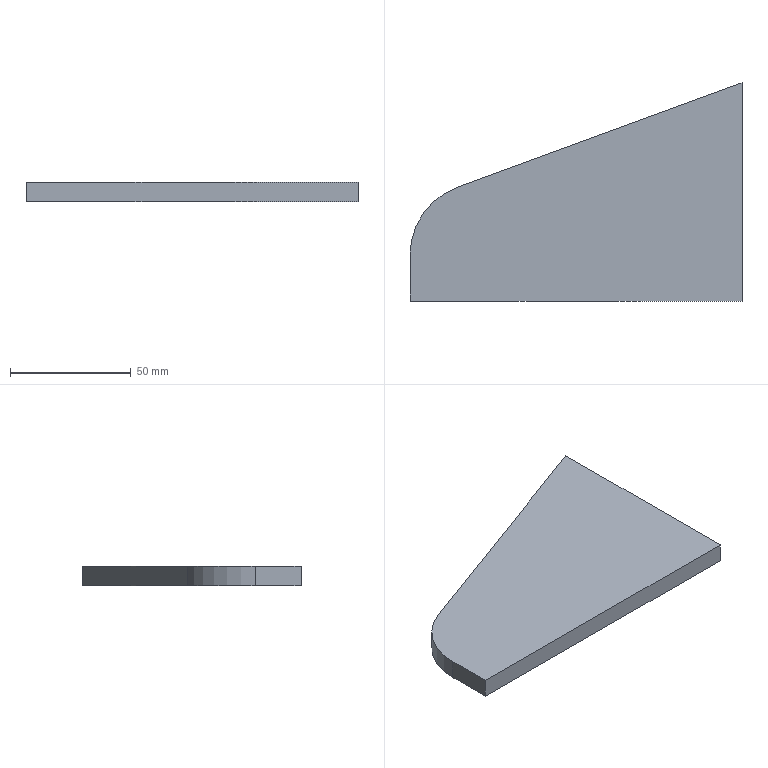Part | SolidWorks | features Extrusion 1 | 1 solid | 7 faces | box 137.522 x 90.425 x 8 mm | volume 71106 mm3 | plane 6 | cylinder 1 | commonest cylinder face diameters 60 x1
STEP:
#1=CARTESIAN_POINT('',(58.628,240.213,0.));
#2=VERTEX_POINT('',#1);
#3=CARTESIAN_POINT('',(38.956,212.047,0.));
#4=VERTEX_POINT('',#3);
#5=CARTESIAN_POINT('',(68.956,212.047,0.));
#6=DIRECTION('',(0.,0.,1.));
#7=DIRECTION('',(1.,0.,0.));
#8=AXIS2_PLACEMENT_3D('',#5,#6,#7);
#9=CIRCLE('',#8,30.);
#10=EDGE_CURVE('',#2,#4,#9,.T.);
#11=ORIENTED_EDGE('',*,*,#10,.T.);
#12=CARTESIAN_POINT('',(38.956,212.047,8.));
#13=VERTEX_POINT('',#12);
#14=CARTESIAN_POINT('',(38.956,212.047,8.));
#15=DIRECTION('',(0.,0.,-1.));
#16=VECTOR('',#15,1000.);
#17=LINE('',#14,#16);
#18=EDGE_CURVE('',#13,#4,#17,.T.);
#19=ORIENTED_EDGE('',*,*,#18,.F.);
#20=CARTESIAN_POINT('',(58.628,240.213,8.));
#21=VERTEX_POINT('',#20);
#22=CARTESIAN_POINT('',(68.956,212.047,8.));
#23=DIRECTION('',(0.,0.,1.));
#24=DIRECTION('',(1.,0.,0.));
#25=AXIS2_PLACEMENT_3D('',#22,#23,#24);
#26=CIRCLE('',#25,30.);
#27=EDGE_CURVE('',#21,#13,#26,.T.);
#28=ORIENTED_EDGE('',*,*,#27,.F.);
#29=CARTESIAN_POINT('',(58.628,240.213,8.));
#30=DIRECTION('',(0.,0.,-1.));
#31=VECTOR('',#30,1000.);
#32=LINE('',#29,#31);
#33=EDGE_CURVE('',#21,#2,#32,.T.);
#34=ORIENTED_EDGE('',*,*,#33,.T.);
#35=EDGE_LOOP('',(#11,#19,#28,#34));
#36=FACE_OUTER_BOUND('',#35,.T.);
#37=CARTESIAN_POINT('',(68.956,212.047,8.));
#38=DIRECTION('',(0.,0.,-1.));
#39=DIRECTION('',(-1.,0.,0.));
#40=AXIS2_PLACEMENT_3D('',#37,#38,#39);
#41=CYLINDRICAL_SURFACE('',#40,30.);
#42=ADVANCED_FACE('',(#36),#41,.T.);
#43=CARTESIAN_POINT('',(38.956,193.,0.));
#44=VERTEX_POINT('',#43);
#45=CARTESIAN_POINT('',(38.956,212.047,0.));
#46=DIRECTION('',(0.,-1.,0.));
#47=VECTOR('',#46,1000.);
#48=LINE('',#45,#47);
#49=EDGE_CURVE('',#4,#44,#48,.T.);
#50=ORIENTED_EDGE('',*,*,#49,.T.);
#51=CARTESIAN_POINT('',(38.956,193.,8.));
#52=VERTEX_POINT('',#51);
#53=CARTESIAN_POINT('',(38.956,193.,8.));
#54=DIRECTION('',(0.,0.,-1.));
#55=VECTOR('',#54,1000.);
#56=LINE('',#53,#55);
#57=EDGE_CURVE('',#52,#44,#56,.T.);
#58=ORIENTED_EDGE('',*,*,#57,.F.);
#59=CARTESIAN_POINT('',(38.956,212.047,8.));
#60=DIRECTION('',(0.,-1.,0.));
#61=VECTOR('',#60,1000.);
#62=LINE('',#59,#61);
#63=EDGE_CURVE('',#13,#52,#62,.T.);
#64=ORIENTED_EDGE('',*,*,#63,.F.);
#65=ORIENTED_EDGE('',*,*,#18,.T.);
#66=EDGE_LOOP('',(#50,#58,#64,#65));
#67=FACE_OUTER_BOUND('',#66,.T.);
#68=CARTESIAN_POINT('',(38.956,212.047,8.));
#69=DIRECTION('',(1.,0.,0.));
#70=DIRECTION('',(0.,1.,0.));
#71=AXIS2_PLACEMENT_3D('',#68,#69,#70);
#72=PLANE('',#71);
#73=ADVANCED_FACE('',(#67),#72,.F.);
#74=CARTESIAN_POINT('',(176.478,193.,0.));
#75=VERTEX_POINT('',#74);
#76=CARTESIAN_POINT('',(38.956,193.,0.));
#77=DIRECTION('',(1.,0.,0.));
#78=VECTOR('',#77,1000.);
#79=LINE('',#76,#78);
#80=EDGE_CURVE('',#44,#75,#79,.T.);
#81=ORIENTED_EDGE('',*,*,#80,.T.);
#82=CARTESIAN_POINT('',(176.478,193.,8.));
#83=VERTEX_POINT('',#82);
#84=CARTESIAN_POINT('',(176.478,193.,8.));
#85=DIRECTION('',(0.,0.,-1.));
#86=VECTOR('',#85,1000.);
#87=LINE('',#84,#86);
#88=EDGE_CURVE('',#83,#75,#87,.T.);
#89=ORIENTED_EDGE('',*,*,#88,.F.);
#90=CARTESIAN_POINT('',(38.956,193.,8.));
#91=DIRECTION('',(1.,0.,0.));
#92=VECTOR('',#91,1000.);
#93=LINE('',#90,#92);
#94=EDGE_CURVE('',#52,#83,#93,.T.);
#95=ORIENTED_EDGE('',*,*,#94,.F.);
#96=ORIENTED_EDGE('',*,*,#57,.T.);
#97=EDGE_LOOP('',(#81,#89,#95,#96));
#98=FACE_OUTER_BOUND('',#97,.T.);
#99=CARTESIAN_POINT('',(38.956,193.,8.));
#100=DIRECTION('',(0.,1.,0.));
#101=DIRECTION('',(-1.,0.,0.));
#102=AXIS2_PLACEMENT_3D('',#99,#100,#101);
#103=PLANE('',#102);
#104=ADVANCED_FACE('',(#98),#103,.F.);
#105=CARTESIAN_POINT('',(176.478,283.425,0.));
#106=VERTEX_POINT('',#105);
#107=CARTESIAN_POINT('',(176.478,283.425,0.));
#108=DIRECTION('',(0.,1.,0.));
#109=VECTOR('',#108,1000.);
#110=LINE('',#107,#109);
#111=EDGE_CURVE('',#75,#106,#110,.T.);
#112=ORIENTED_EDGE('',*,*,#111,.T.);
#113=CARTESIAN_POINT('',(176.478,283.425,8.));
#114=VERTEX_POINT('',#113);
#115=CARTESIAN_POINT('',(176.478,283.425,8.));
#116=DIRECTION('',(0.,0.,-1.));
#117=VECTOR('',#116,1000.);
#118=LINE('',#115,#117);
#119=EDGE_CURVE('',#114,#106,#118,.T.);
#120=ORIENTED_EDGE('',*,*,#119,.F.);
#121=CARTESIAN_POINT('',(176.478,283.425,8.));
#122=DIRECTION('',(0.,1.,0.));
#123=VECTOR('',#122,1000.);
#124=LINE('',#121,#123);
#125=EDGE_CURVE('',#83,#114,#124,.T.);
#126=ORIENTED_EDGE('',*,*,#125,.F.);
#127=ORIENTED_EDGE('',*,*,#88,.T.);
#128=EDGE_LOOP('',(#112,#120,#126,#127));
#129=FACE_OUTER_BOUND('',#128,.T.);
#130=CARTESIAN_POINT('',(176.478,283.425,8.));
#131=DIRECTION('',(-1.,0.,0.));
#132=DIRECTION('',(0.,0.,1.));
#133=AXIS2_PLACEMENT_3D('',#130,#131,#132);
#134=PLANE('',#133);
#135=ADVANCED_FACE('',(#129),#134,.F.);
#136=CARTESIAN_POINT('',(176.478,283.425,0.));
#137=DIRECTION('',(-0.9389,-0.3443,0.));
#138=VECTOR('',#137,1000.);
#139=LINE('',#136,#138);
#140=EDGE_CURVE('',#106,#2,#139,.T.);
#141=ORIENTED_EDGE('',*,*,#140,.T.);
#142=ORIENTED_EDGE('',*,*,#33,.F.);
#143=CARTESIAN_POINT('',(176.478,283.425,8.));
#144=DIRECTION('',(-0.9389,-0.3443,0.));
#145=VECTOR('',#144,1000.);
#146=LINE('',#143,#145);
#147=EDGE_CURVE('',#114,#21,#146,.T.);
#148=ORIENTED_EDGE('',*,*,#147,.F.);
#149=ORIENTED_EDGE('',*,*,#119,.T.);
#150=EDGE_LOOP('',(#141,#142,#148,#149));
#151=FACE_OUTER_BOUND('',#150,.T.);
#152=CARTESIAN_POINT('',(176.478,283.425,8.));
#153=DIRECTION('',(0.3443,-0.9389,0.));
#154=DIRECTION('',(0.9389,0.3443,0.));
#155=AXIS2_PLACEMENT_3D('',#152,#153,#154);
#156=PLANE('',#155);
#157=ADVANCED_FACE('',(#151),#156,.F.);
#158=ORIENTED_EDGE('',*,*,#27,.T.);
#159=ORIENTED_EDGE('',*,*,#63,.T.);
#160=ORIENTED_EDGE('',*,*,#94,.T.);
#161=ORIENTED_EDGE('',*,*,#125,.T.);
#162=ORIENTED_EDGE('',*,*,#147,.T.);
#163=EDGE_LOOP('',(#158,#159,#160,#161,#162));
#164=FACE_OUTER_BOUND('',#163,.T.);
#165=CARTESIAN_POINT('',(68.956,212.047,8.));
#166=DIRECTION('',(0.,0.,1.));
#167=DIRECTION('',(1.,0.,0.));
#168=AXIS2_PLACEMENT_3D('',#165,#166,#167);
#169=PLANE('',#168);
#170=ADVANCED_FACE('',(#164),#169,.T.);
#171=ORIENTED_EDGE('',*,*,#10,.F.);
#172=ORIENTED_EDGE('',*,*,#140,.F.);
#173=ORIENTED_EDGE('',*,*,#111,.F.);
#174=ORIENTED_EDGE('',*,*,#80,.F.);
#175=ORIENTED_EDGE('',*,*,#49,.F.);
#176=EDGE_LOOP('',(#171,#172,#173,#174,#175));
#177=FACE_OUTER_BOUND('',#176,.T.);
#178=CARTESIAN_POINT('',(68.956,212.047,0.));
#179=DIRECTION('',(0.,0.,1.));
#180=DIRECTION('',(1.,0.,0.));
#181=AXIS2_PLACEMENT_3D('',#178,#179,#180);
#182=PLANE('',#181);
#183=ADVANCED_FACE('',(#177),#182,.F.);
#184=CLOSED_SHELL('',(#42,#73,#104,#135,#157,#170,#183));
#185=MANIFOLD_SOLID_BREP('',#184);
#186=CARTESIAN_POINT('',(0.,0.,0.));
#187=DIRECTION('',(0.,0.,1.));
#188=DIRECTION('',(1.,0.,0.));
#189=AXIS2_PLACEMENT_3D('',#186,#187,#188);
#190=(LENGTH_UNIT()NAMED_UNIT(*)SI_UNIT(.MILLI.,.METRE.));
#191=UNCERTAINTY_MEASURE_WITH_UNIT(LENGTH_MEASURE(0.00001),#190,'','');
#192=(NAMED_UNIT(*)PLANE_ANGLE_UNIT()SI_UNIT($,.RADIAN.));
#193=(NAMED_UNIT(*)SI_UNIT($,.STERADIAN.)SOLID_ANGLE_UNIT());
#194=(GEOMETRIC_REPRESENTATION_CONTEXT(3)GLOBAL_UNCERTAINTY_ASSIGNED_CONTEXT((#191))GLOBAL_UNIT_ASSIGNED_CONTEXT((#190,#192,#193))REPRESENTATION_CONTEXT('',''));
#195=ADVANCED_BREP_SHAPE_REPRESENTATION('',(#185,#189),#194);